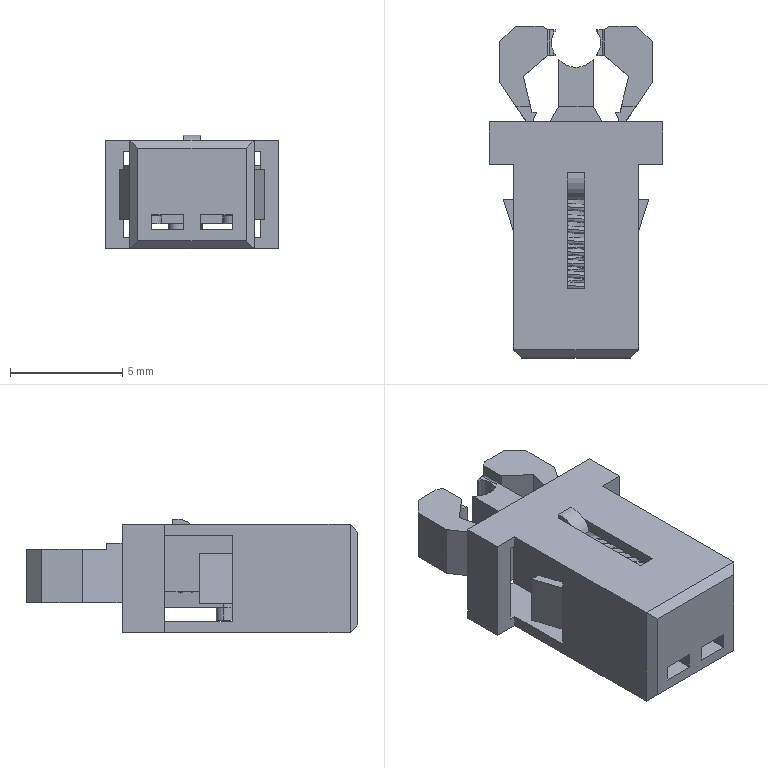Part | SolidWorks | 4 solids | 201 faces | box 7.7 x 14.77 x 5.058 mm | volume 193.431 mm3 | plane 163 | cylinder 34 | cone 2 | spline 2 | commonest cylinder face diameters 0.91 x6 1.4 x5 0.14 x4 0.42 x3 0.77 x3 0.84 x3